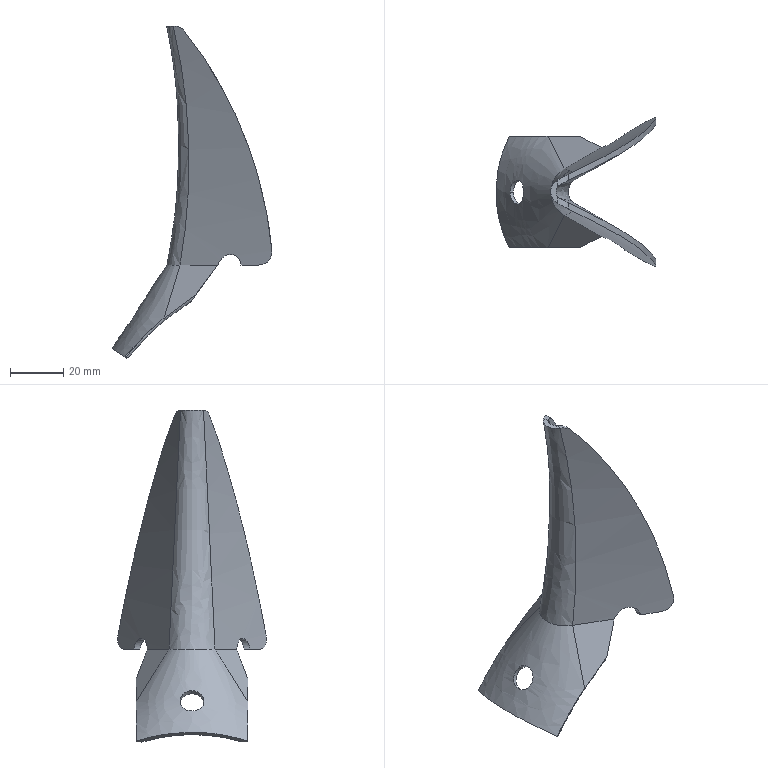Part | NX | features BREP 1 | 1 solid | 36 faces | box 60.225 x 56.002 x 125 mm | volume 14163 mm3 | cylinder 16 | plane 14 | spline 6 | commonest cylinder face diameters 8 x4 10 x4 9 x2 314.344 x2 895.773 x2 895.783 x2